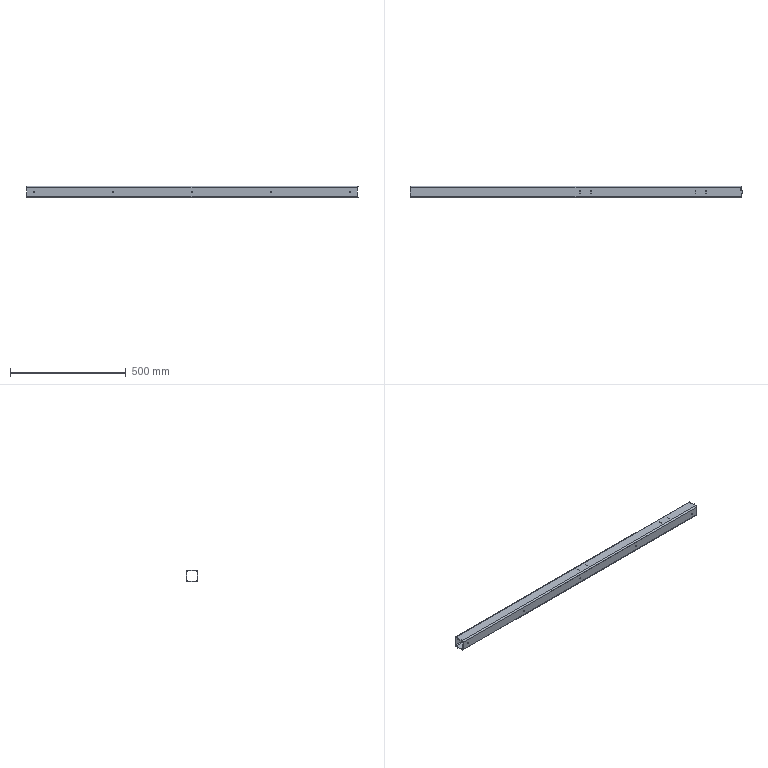Part | SolidWorks | features BaseBody 1 | 1 solid | 107 faces | box 1436 x 50 x 50 mm | volume 773039 mm3 | plane 63 | spline 25 | cylinder 19 | commonest cylinder face diameters 4.2 x10 6 x4 12 x4 8 x1